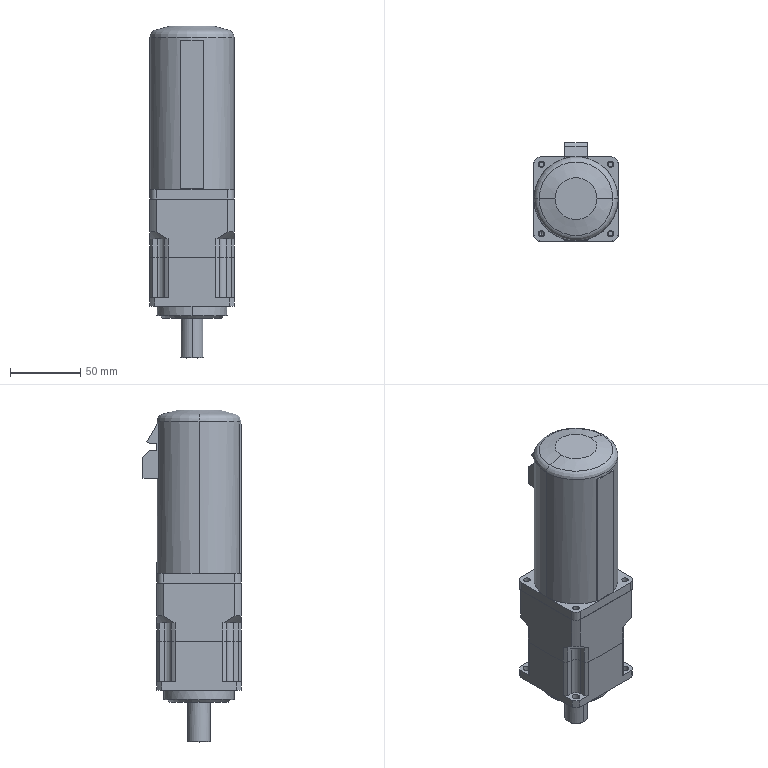Part | NX | 3 solids | 223 faces | box 60 x 70 x 237 mm | volume 578029 mm3 | cylinder 96 | plane 95 | cone 22 | torus 10 | commonest cylinder face diameters 69 x16 10 x12 3.3 x8 4.5 x8 5.5 x8 50 x6